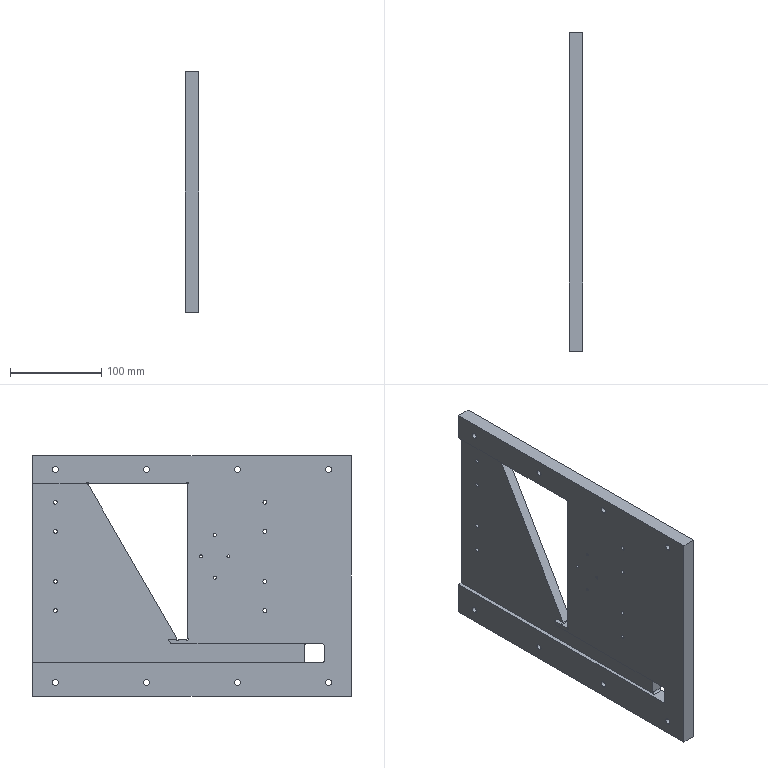Part | STEP file | 02-19 Separating mechanism seal plate | 1 solid | 94 faces | box 15 x 350 x 264 mm | volume 1110870 mm3 | cylinder 68 | plane 26 | commonest cylinder face diameters 4.2 x16 6.5 x16 12 x16 2 x8 3.3 x8 4 x4